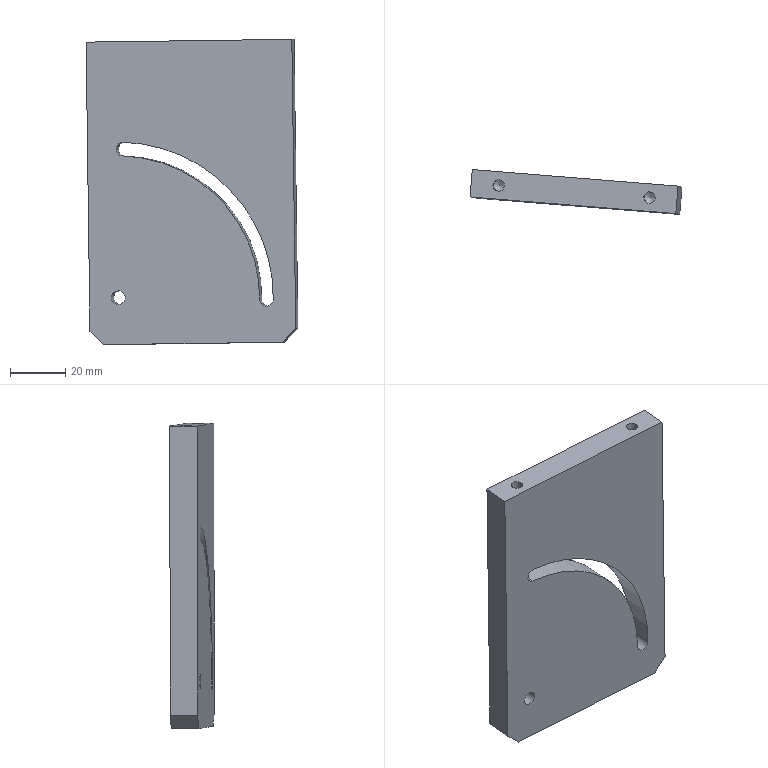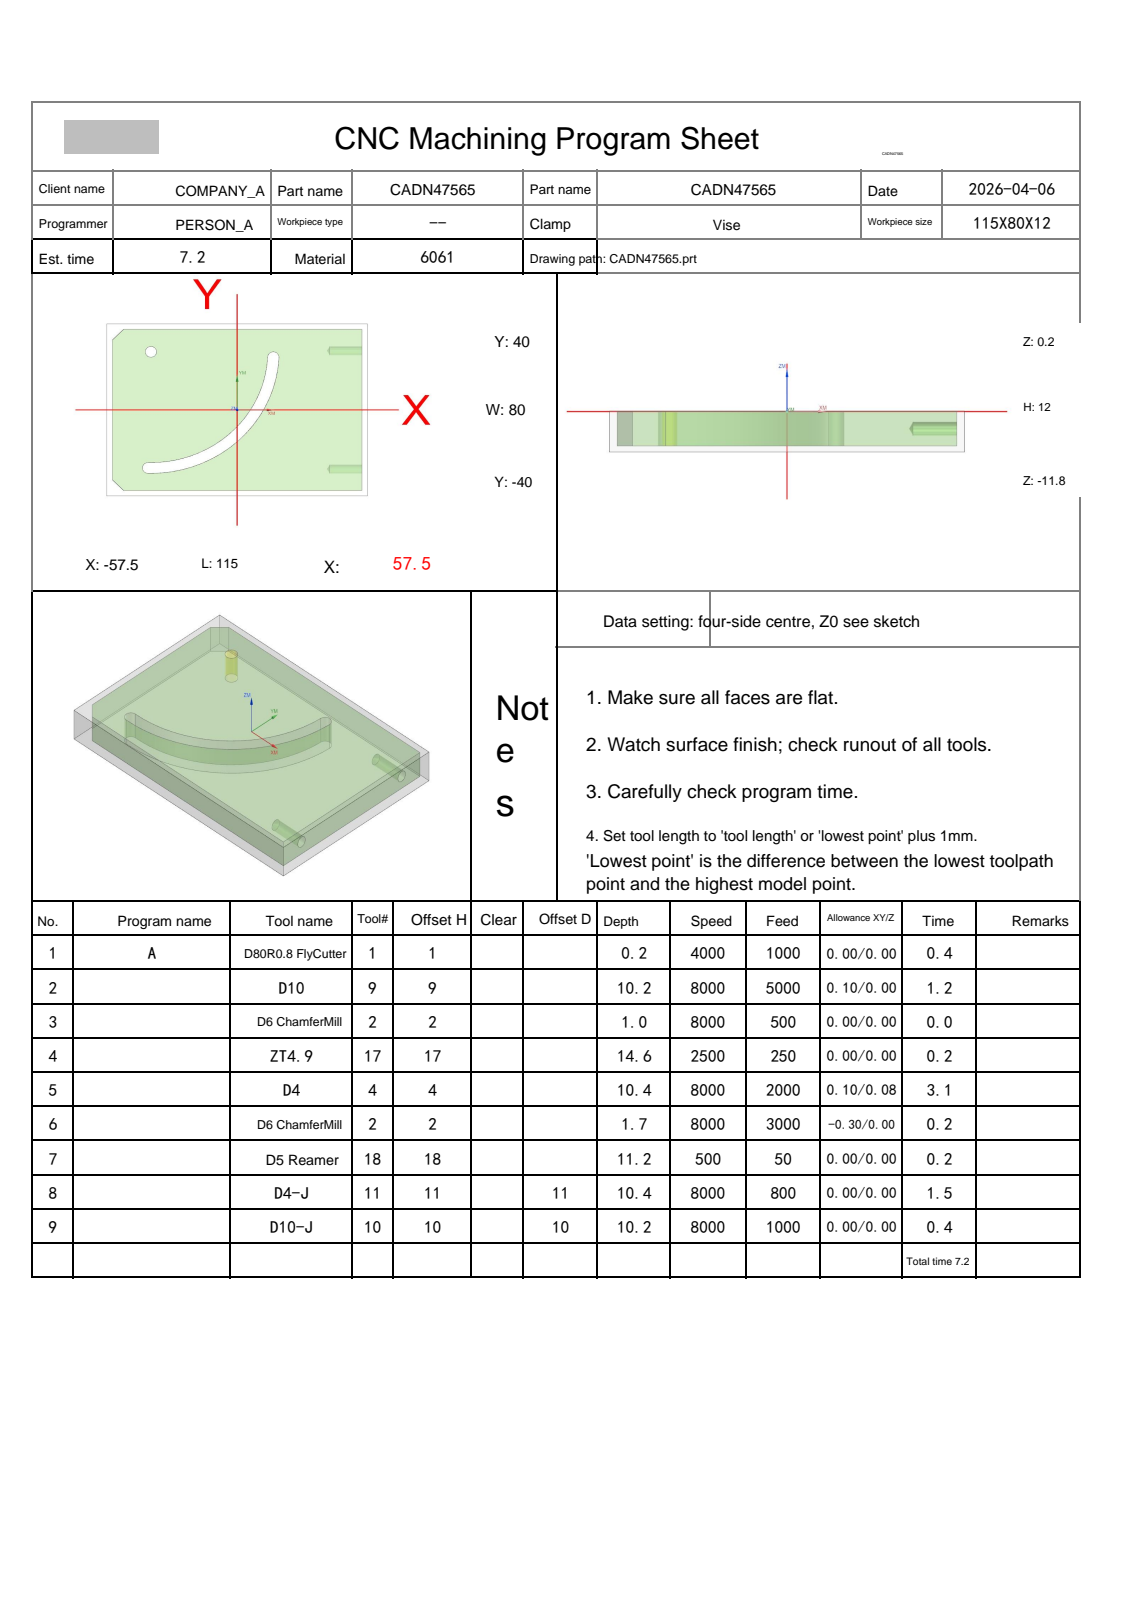NC program | NX | posted by the shop | part box 76.959 x 16.139 x 110.936 mm
Whole program:
%
O0001
(Machine time: 9.16 MIN)
(===Total Tool:8===)
(T1=D80R0.8 FlyCutter D=80.  R=0.8  D-  H01 Z=0.    )
(T9=D10     D=10.  R=0.   D-  H09 Z=-10.  )
(T2=D6 ChamferMill D=6.   R=0.   D-  H02 Z=-1.5  )
(T17=ZT4.9  D=4.9  DR_a=120 D-  H17 Z=-14.41)
(T4=D4      D=4.   R=0.   D-  H04 Z=-10.2 )
(T18=D5 Reamer D=5.   DR_a=180 D-  H18 Z=-11.  )
(T11=D4-J   D=4.   R=0.   D11 H11 Z=-10.2 )
(T10=D10-J  D=10.  R=0.   D10 H10 Z=-10.  )
G80 G90 G17 G49 G40
G91 G28 Z0
M01
N1 T01 M06
(D80R0.8 FlyCutter D=80. R=0.8 H=01 ce=0.00 di=0.00)
(MAX_Z=20. MIN_Z=0. Time=0.46M)
G00 G90 G54 X-100. Y25.833 M03 S4000
G43 H01 Z20.
M08
Z2.
G01 Z0.0 F1000.
X-95.
X95.
Y-25.833
X-95.
X-100.
Z2.
G00 Z20.
G91 G28 Z0.0
M05
M09
G91 G28 Z0.0
M01
N2 T09 M06
(D10  D=10. R=0. H=09 ce=0.10 di=0.00)
(MAX_Z=20. MIN_Z=-10. Time=1.20M)
G00 G90 G54 X2.5 Y42.6 M03 S8000
G43 H09 Z20.
M08
Z.5
G01 X55. Z.401 F5000.
G02 X60.1 Y37.5 Z.385 I0.0 J-5.1
G01 Y-37.5 Z.243
G02 X55. Y-42.6 Z.228 I-5.1 J0.0
G01 X-50. Z.03
G02 X-53.606 Y-41.106 Z.022 I0.0 J5.1
G01 X-58.606 Y-36.106 Z.009
G02 X-60.1 Y-32.5 Z.001 I3.606 J3.606
G01 Y32.5 Z-.122
G02 X-58.606 Y36.106 Z-.13 I5.1 J0.0
G01 X-53.606 Y41.106 Z-.143
G02 X-50. Y42.6 Z-.151 I3.606 J-3.606
G01 X55. Z-.349
G02 X60.1 Y37.5 Z-.365 I0.0 J-5.1
G01 Y-37.5 Z-.507
G02 X55. Y-42.6 Z-.522 I-5.1 J0.0
G01 X-50. Z-.72
G02 X-53.606 Y-41.106 Z-.728 I0.0 J5.1
G01 X-58.606 Y-36.106 Z-.741
G02 X-60.1 Y-32.5 Z-.749 I3.606 J3.606
G01 Y32.5 Z-.872
G02 X-58.606 Y36.106 Z-.88 I5.1 J0.0
G01 X-53.606 Y41.106 Z-.893
G02 X-50. Y42.6 Z-.901 I3.606 J-3.606
G01 X55. Z-1.099
G02 X60.1 Y37.5 Z-1.115 I0.0 J-5.1
G01 Y-37.5 Z-1.257
G02 X55. Y-42.6 Z-1.272 I-5.1 J0.0
G01 X-50. Z-1.47
G02 X-53.606 Y-41.106 Z-1.478 I0.0 J5.1
G01 X-58.606 Y-36.106 Z-1.491
G02 X-60.1 Y-32.5 Z-1.499 I3.606 J3.606
G01 Y32.5 Z-1.622
G02 X-58.606 Y36.106 Z-1.63 I5.1 J0.0
G01 X-53.606 Y41.106 Z-1.643
G02 X-50. Y42.6 Z-1.651 I3.606 J-3.606
G01 X55. Z-1.849
G02 X60.1 Y37.5 Z-1.865 I0.0 J-5.1
G01 Y-37.5 Z-2.007
G02 X55. Y-42.6 Z-2.022 I-5.1 J0.0
G01 X-50. Z-2.22
G02 X-53.606 Y-41.106 Z-2.228 I0.0 J5.1
G01 X-58.606 Y-36.106 Z-2.241
G02 X-60.1 Y-32.5 Z-2.249 I3.606 J3.606
G01 Y32.5 Z-2.372
G02 X-58.606 Y36.106 Z-2.38 I5.1 J0.0
G01 X-53.606 Y41.106 Z-2.393
G02 X-50. Y42.6 Z-2.401 I3.606 J-3.606
G01 X55. Z-2.599
G02 X60.1 Y37.5 Z-2.615 I0.0 J-5.1
G01 Y-37.5 Z-2.757
G02 X55. Y-42.6 Z-2.772 I-5.1 J0.0
G01 X-50. Z-2.97
G02 X-53.606 Y-41.106 Z-2.978 I0.0 J5.1
G01 X-58.606 Y-36.106 Z-2.991
G02 X-60.1 Y-32.5 Z-2.999 I3.606 J3.606
G01 Y32.5 Z-3.122
G02 X-58.606 Y36.106 Z-3.13 I5.1 J0.0
G01 X-53.606 Y41.106 Z-3.143
G02 X-50. Y42.6 Z-3.151 I3.606 J-3.606
G01 X55. Z-3.349
G02 X60.1 Y37.5 Z-3.365 I0.0 J-5.1
G01 Y-37.5 Z-3.507
G02 X55. Y-42.6 Z-3.522 I-5.1 J0.0
G01 X-50. Z-3.72
G02 X-53.606 Y-41.106 Z-3.728 I0.0 J5.1
G01 X-58.606 Y-36.106 Z-3.741
G02 X-60.1 Y-32.5 Z-3.749 I3.606 J3.606
G01 Y32.5 Z-3.872
G02 X-58.606 Y36.106 Z-3.88 I5.1 J0.0
G01 X-53.606 Y41.106 Z-3.893
G02 X-50. Y42.6 Z-3.901 I3.606 J-3.606
G01 X55. Z-4.099
G02 X60.1 Y37.5 Z-4.115 I0.0 J-5.1
G01 Y-37.5 Z-4.257
G02 X55. Y-42.6 Z-4.272 I-5.1 J0.0
G01 X-50. Z-4.47
G02 X-53.606 Y-41.106 Z-4.478 I0.0 J5.1
G01 X-58.606 Y-36.106 Z-4.491
G02 X-60.1 Y-32.5 Z-4.499 I3.606 J3.606
G01 Y32.5 Z-4.622
G02 X-58.606 Y36.106 Z-4.63 I5.1 J0.0
G01 X-53.606 Y41.106 Z-4.643
G02 X-50. Y42.6 Z-4.651 I3.606 J-3.606
G01 X55. Z-4.849
G02 X60.1 Y37.5 Z-4.865 I0.0 J-5.1
G01 Y-37.5 Z-5.007
G02 X55. Y-42.6 Z-5.022 I-5.1 J0.0
G01 X-50. Z-5.22
G02 X-53.606 Y-41.106 Z-5.228 I0.0 J5.1
G01 X-58.606 Y-36.106 Z-5.241
G02 X-60.1 Y-32.5 Z-5.249 I3.606 J3.606
G01 Y32.5 Z-5.372
G02 X-58.606 Y36.106 Z-5.38 I5.1 J0.0
G01 X-53.606 Y41.106 Z-5.393
G02 X-50. Y42.6 Z-5.401 I3.606 J-3.606
G01 X55. Z-5.599
G02 X60.1 Y37.5 Z-5.615 I0.0 J-5.1
G01 Y-37.5 Z-5.757
G02 X55. Y-42.6 Z-5.772 I-5.1 J0.0
G01 X-50. Z-5.97
G02 X-53.606 Y-41.106 Z-5.978 I0.0 J5.1
G01 X-58.606 Y-36.106 Z-5.991
G02 X-60.1 Y-32.5 Z-5.999 I3.606 J3.606
G01 Y32.5 Z-6.122
G02 X-58.606 Y36.106 Z-6.13 I5.1 J0.0
G01 X-53.606 Y41.106 Z-6.143
G02 X-50. Y42.6 Z-6.151 I3.606 J-3.606
G01 X55. Z-6.349
G02 X60.1 Y37.5 Z-6.365 I0.0 J-5.1
G01 Y-37.5 Z-6.507
G02 X55. Y-42.6 Z-6.522 I-5.1 J0.0
G01 X-50. Z-6.72
G02 X-53.606 Y-41.106 Z-6.728 I0.0 J5.1
G01 X-58.606 Y-36.106 Z-6.741
G02 X-60.1 Y-32.5 Z-6.749 I3.606 J3.606
G01 Y32.5 Z-6.872
G02 X-58.606 Y36.106 Z-6.88 I5.1 J0.0
G01 X-53.606 Y41.106 Z-6.893
G02 X-50. Y42.6 Z-6.901 I3.606 J-3.606
G01 X55. Z-7.099
G02 X60.1 Y37.5 Z-7.115 I0.0 J-5.1
G01 Y-37.5 Z-7.257
G02 X55. Y-42.6 Z-7.272 I-5.1 J0.0
G01 X-50. Z-7.47
G02 X-53.606 Y-41.106 Z-7.478 I0.0 J5.1
G01 X-58.606 Y-36.106 Z-7.491
G02 X-60.1 Y-32.5 Z-7.499 I3.606 J3.606
G01 Y32.5 Z-7.622
G02 X-58.606 Y36.106 Z-7.63 I5.1 J0.0
G01 X-53.606 Y41.106 Z-7.643
G02 X-50. Y42.6 Z-7.651 I3.606 J-3.606
G01 X55. Z-7.849
G02 X60.1 Y37.5 Z-7.865 I0.0 J-5.1
G01 Y-37.5 Z-8.007
G02 X55. Y-42.6 Z-8.022 I-5.1 J0.0
G01 X-50. Z-8.22
G02 X-53.606 Y-41.106 Z-8.228 I0.0 J5.1
G01 X-58.606 Y-36.106 Z-8.241
G02 X-60.1 Y-32.5 Z-8.249 I3.606 J3.606
G01 Y32.5 Z-8.372
G02 X-58.606 Y36.106 Z-8.38 I5.1 J0.0
G01 X-53.606 Y41.106 Z-8.393
G02 X-50. Y42.6 Z-8.401 I3.606 J-3.606
G01 X55. Z-8.599
G02 X60.1 Y37.5 Z-8.615 I0.0 J-5.1
G01 Y-37.5 Z-8.757
G02 X55. Y-42.6 Z-8.772 I-5.1 J0.0
G01 X-50. Z-8.97
G02 X-53.606 Y-41.106 Z-8.978 I0.0 J5.1
G01 X-58.606 Y-36.106 Z-8.991
G02 X-60.1 Y-32.5 Z-8.999 I3.606 J3.606
G01 Y32.5 Z-9.122
G02 X-58.606 Y36.106 Z-9.13 I5.1 J0.0
G01 X-53.606 Y41.106 Z-9.143
G02 X-50. Y42.6 Z-9.151 I3.606 J-3.606
G01 X55. Z-9.349
G02 X60.1 Y37.5 Z-9.365 I0.0 J-5.1
G01 Y-37.5 Z-9.507
G02 X55. Y-42.6 Z-9.522 I-5.1 J0.0
G01 X-50. Z-9.72
G02 X-53.606 Y-41.106 Z-9.728 I0.0 J5.1
G01 X-58.606 Y-36.106 Z-9.741
G02 X-60.1 Y-32.5 Z-9.749 I3.606 J3.606
G01 Y32.5 Z-9.872
G02 X-58.606 Y36.106 Z-9.88 I5.1 J0.0
G01 X-53.606 Y41.106 Z-9.893
G02 X-50. Y42.6 Z-9.901 I3.606 J-3.606
G01 X2.5 Z-10.
X55.
G02 X60.1 Y37.5 I0.0 J-5.1
G01 Y-37.5
G02 X55. Y-42.6 I-5.1 J0.0
G01 X-50.
G02 X-53.606 Y-41.106 I0.0 J5.1
G01 X-58.606 Y-36.106
G02 X-60.1 Y-32.5 I3.606 J3.606
G01 Y32.5
G02 X-58.606 Y36.106 I5.1 J0.0
G01 X-53.606 Y41.106
G02 X-50. Y42.6 I3.606 J-3.606
G01 X2.5
X3.
Z-9.
G00 Z20.
G91 G28 Z0.0
M05
M09
G91 G28 Z0.0
M01
N3 T02 M06
(D6 ChamferMill D=6. R=0. H=02 ce=0.00 di=0.00)
(MAX_Z=20. MIN_Z=-0.8 Time=0.03M)
G00 G90 G54 X-38. Y27. M03 S8000
G43 H02 Z20.
M08
G98 G81 X-38. Y27. Z-.8 R1. F500.
X-39.287 Y-26.985
X15.942 Y24.5
G80
G00 Z20.
G91 G28 Z0.0
M05
M09
G91 G28 Z0.0
M01
N4 T17 M06
(ZT4.9 D=4.9 DR_a=120 H=17)
(MAX_Z=20. MIN_Z=-14.41 Time=0.20M)
G00 G90 G54 X-38. Y27. M03 S2500
G43 H17 Z20.
M08
G98 G83 X-38. Y27. Z-14.415 R1. F250. Q2.
X-39.287 Y-26.985
X15.942 Y24.5
G80
G00 Z20.
G91 G28 Z0.0
M05
M09
G91 G28 Z0.0
M01
N5 T04 M06
(D4  D=4. R=0. H=04 ce=0.10 di=0.08)
(MAX_Z=20. MIN_Z=-10.2 Time=3.07M)
G00 G90 G54 X-25.456 Y-25.084 M03 S8000
G43 H04 Z20.
M08
Z.8
G01 X-27.62 Y-25.616 Z.683 F2000.
X-32.529 Y-26.35 Z.423
X-37.485 Y-26.628 Z.163
X-39.278 Y-26.585 Z.069
X-39.436 Y-26.581 Z.061
X-39.683 Y-26.817 Z.043
X-39.687 Y-26.975 Z.034
X-39.691 Y-27.133 Z.026
X-39.455 Y-27.381 Z.008
X-39.297 Y-27.385 Z0.0
G03 X16.342 Y24.481 Z-.145 I1.297 J54.385
X16.2 Y24.805 Z-.145 I-.4 J.019
X15.961 Y24.899 Z-.146 I-.258 J-.306
X15.543 Y24.518 Z-.147 I-.019 J-.4
G02 X-39.278 Y-26.585 Z-.289 I-53.543 J2.482
G03 X-39.687 Y-26.975 Z-.29 I-.01 J-.4
X-39.297 Y-27.385 Z-.291 I.4 J-.01
X16.342 Y24.481 Z-.436 I1.297 J54.385
X16.2 Y24.805 Z-.437 I-.4 J.019
X15.961 Y24.899 Z-.437 I-.258 J-.306
X15.543 Y24.518 Z-.438 I-.019 J-.4
G02 X-39.278 Y-26.585 Z-.581 I-53.543 J2.482
G03 X-39.687 Y-26.975 Z-.582 I-.01 J-.4
X-39.297 Y-27.385 Z-.583 I.4 J-.01
X16.342 Y24.481 Z-.727 I1.297 J54.385
X16.2 Y24.805 Z-.728 I-.4 J.019
X15.961 Y24.899 Z-.729 I-.258 J-.306
X15.543 Y24.518 Z-.73 I-.019 J-.4
G02 X-39.278 Y-26.585 Z-.872 I-53.543 J2.482
G03 X-39.687 Y-26.975 Z-.873 I-.01 J-.4
X-39.297 Y-27.385 Z-.874 I.4 J-.01
X16.342 Y24.481 Z-1.019 I1.297 J54.385
X16.2 Y24.805 Z-1.02 I-.4 J.019
X15.961 Y24.899 Z-1.02 I-.258 J-.306
X15.543 Y24.518 Z-1.021 I-.019 J-.4
G02 X-39.278 Y-26.585 Z-1.164 I-53.543 J2.482
G03 X-39.687 Y-26.975 Z-1.165 I-.01 J-.4
X-39.297 Y-27.385 Z-1.166 I.4 J-.01
X16.342 Y24.481 Z-1.31 I1.297 J54.385
X16.2 Y24.805 Z-1.311 I-.4 J.019
X15.961 Y24.899 Z-1.311 I-.258 J-.306
X15.543 Y24.518 Z-1.312 I-.019 J-.4
G02 X-39.278 Y-26.585 Z-1.455 I-53.543 J2.482
G03 X-39.687 Y-26.975 Z-1.456 I-.01 J-.4
X-39.297 Y-27.385 Z-1.457 I.4 J-.01
X16.342 Y24.481 Z-1.602 I1.297 J54.385
X16.2 Y24.805 Z-1.602 I-.4 J.019
X15.961 Y24.899 Z-1.603 I-.258 J-.306
X15.543 Y24.518 Z-1.604 I-.019 J-.4
G02 X-39.278 Y-26.585 Z-1.746 I-53.543 J2.482
G03 X-39.687 Y-26.975 Z-1.747 I-.01 J-.4
X-39.297 Y-27.385 Z-1.749 I.4 J-.01
X16.342 Y24.481 Z-1.893 I1.297 J54.385
X16.2 Y24.805 Z-1.894 I-.4 J.019
X15.961 Y24.899 Z-1.894 I-.258 J-.306
X15.543 Y24.518 Z-1.895 I-.019 J-.4
G02 X-39.278 Y-26.585 Z-2.038 I-53.543 J2.482
G03 X-39.687 Y-26.975 Z-2.039 I-.01 J-.4
X-39.297 Y-27.385 Z-2.04 I.4 J-.01
X16.342 Y24.481 Z-2.185 I1.297 J54.385
X16.2 Y24.805 Z-2.185 I-.4 J.019
X15.961 Y24.899 Z-2.186 I-.258 J-.306
X15.543 Y24.518 Z-2.187 I-.019 J-.4
G02 X-39.278 Y-26.585 Z-2.329 I-53.543 J2.482
G03 X-39.687 Y-26.975 Z-2.33 I-.01 J-.4
X-39.297 Y-27.385 Z-2.331 I.4 J-.01
X16.342 Y24.481 Z-2.476 I1.297 J54.385
X16.2 Y24.805 Z-2.477 I-.4 J.019
X15.961 Y24.899 Z-2.477 I-.258 J-.306
X15.543 Y24.518 Z-2.478 I-.019 J-.4
G02 X-39.278 Y-26.585 Z-2.621 I-53.543 J2.482
G03 X-39.687 Y-26.975 Z-2.622 I-.01 J-.4
X-39.297 Y-27.385 Z-2.623 I.4 J-.01
X16.342 Y24.481 Z-2.767 I1.297 J54.385
X16.2 Y24.805 Z-2.768 I-.4 J.019
X15.961 Y24.899 Z-2.769 I-.258 J-.306
X15.543 Y24.518 Z-2.77 I-.019 J-.4
G02 X-39.278 Y-26.585 Z-2.912 I-53.543 J2.482
G03 X-39.687 Y-26.975 Z-2.913 I-.01 J-.4
X-39.297 Y-27.385 Z-2.914 I.4 J-.01
X16.342 Y24.481 Z-3.059 I1.297 J54.385
X16.2 Y24.805 Z-3.06 I-.4 J.019
X15.961 Y24.899 Z-3.06 I-.258 J-.306
X15.543 Y24.518 Z-3.061 I-.019 J-.4
G02 X-39.278 Y-26.585 Z-3.204 I-53.543 J2.482
G03 X-39.687 Y-26.975 Z-3.205 I-.01 J-.4
X-39.297 Y-27.385 Z-3.206 I.4 J-.01
X16.342 Y24.481 Z-3.35 I1.297 J54.385
X16.2 Y24.805 Z-3.351 I-.4 J.019
X15.961 Y24.899 Z-3.351 I-.258 J-.306
X15.543 Y24.518 Z-3.352 I-.019 J-.4
G02 X-39.278 Y-26.585 Z-3.495 I-53.543 J2.482
G03 X-39.687 Y-26.975 Z-3.496 I-.01 J-.4
X-39.297 Y-27.385 Z-3.497 I.4 J-.01
X16.342 Y24.481 Z-3.642 I1.297 J54.385
X16.2 Y24.805 Z-3.642 I-.4 J.019
X15.961 Y24.899 Z-3.643 I-.258 J-.306
X15.543 Y24.518 Z-3.644 I-.019 J-.4
G02 X-39.278 Y-26.585 Z-3.786 I-53.543 J2.482
G03 X-39.687 Y-26.975 Z-3.787 I-.01 J-.4
X-39.297 Y-27.385 Z-3.789 I.4 J-.01
X16.342 Y24.481 Z-3.933 I1.297 J54.385
X16.2 Y24.805 Z-3.934 I-.4 J.019
X15.961 Y24.899 Z-3.934 I-.258 J-.306
X15.543 Y24.518 Z-3.935 I-.019 J-.4
G02 X-39.278 Y-26.585 Z-4.078 I-53.543 J2.482
G03 X-39.687 Y-26.975 Z-4.079 I-.01 J-.4
X-39.297 Y-27.385 Z-4.08 I.4 J-.01
X16.342 Y24.481 Z-4.225 I1.297 J54.385
X16.2 Y24.805 Z-4.225 I-.4 J.019
X15.961 Y24.899 Z-4.226 I-.258 J-.306
X15.543 Y24.518 Z-4.227 I-.019 J-.4
G02 X-39.278 Y-26.585 Z-4.369 I-53.543 J2.482
G03 X-39.687 Y-26.975 Z-4.37 I-.01 J-.4
X-39.297 Y-27.385 Z-4.371 I.4 J-.01
X16.342 Y24.481 Z-4.516 I1.297 J54.385
X16.2 Y24.805 Z-4.517 I-.4 J.019
X15.961 Y24.899 Z-4.517 I-.258 J-.306
X15.543 Y24.518 Z-4.518 I-.019 J-.4
G02 X-39.278 Y-26.585 Z-4.661 I-53.543 J2.482
G03 X-39.687 Y-26.975 Z-4.662 I-.01 J-.4
X-39.297 Y-27.385 Z-4.663 I.4 J-.01
X16.342 Y24.481 Z-4.807 I1.297 J54.385
X16.2 Y24.805 Z-4.808 I-.4 J.019
X15.961 Y24.899 Z-4.809 I-.258 J-.306
X15.543 Y24.518 Z-4.81 I-.019 J-.4
G02 X-39.278 Y-26.585 Z-4.952 I-53.543 J2.482
G03 X-39.687 Y-26.975 Z-4.953 I-.01 J-.4
X-39.297 Y-27.385 Z-4.954 I.4 J-.01
X16.342 Y24.481 Z-5.099 I1.297 J54.385
X16.2 Y24.805 Z-5.1 I-.4 J.019
X15.961 Y24.899 Z-5.1 I-.258 J-.306
X15.543 Y24.518 Z-5.101 I-.019 J-.4
G02 X-39.278 Y-26.585 Z-5.244 I-53.543 J2.482
G03 X-39.687 Y-26.975 Z-5.245 I-.01 J-.4
X-39.297 Y-27.385 Z-5.246 I.4 J-.01
X16.342 Y24.481 Z-5.39 I1.297 J54.385
X16.2 Y24.805 Z-5.391 I-.4 J.019
X15.961 Y24.899 Z-5.391 I-.258 J-.306
X15.543 Y24.518 Z-5.392 I-.019 J-.4
G02 X-39.278 Y-26.585 Z-5.535 I-53.543 J2.482
G03 X-39.687 Y-26.975 Z-5.536 I-.01 J-.4
X-39.297 Y-27.385 Z-5.537 I.4 J-.01
X16.342 Y24.481 Z-5.682 I1.297 J54.385
X16.2 Y24.805 Z-5.682 I-.4 J.019
X15.961 Y24.899 Z-5.683 I-.258 J-.306
X15.543 Y24.518 Z-5.684 I-.019 J-.4
G02 X-39.278 Y-26.585 Z-5.826 I-53.543 J2.482
G03 X-39.687 Y-26.975 Z-5.827 I-.01 J-.4
X-39.297 Y-27.385 Z-5.829 I.4 J-.01
X16.342 Y24.481 Z-5.973 I1.297 J54.385
X16.2 Y24.805 Z-5.974 I-.4 J.019
X15.961 Y24.899 Z-5.974 I-.258 J-.306
X15.543 Y24.518 Z-5.975 I-.019 J-.4
G02 X-39.278 Y-26.585 Z-6.118 I-53.543 J2.482
G03 X-39.687 Y-26.975 Z-6.119 I-.01 J-.4
X-39.297 Y-27.385 Z-6.12 I.4 J-.01
X16.342 Y24.481 Z-6.265 I1.297 J54.385
X16.2 Y24.805 Z-6.265 I-.4 J.019
X15.961 Y24.899 Z-6.266 I-.258 J-.306
X15.543 Y24.518 Z-6.267 I-.019 J-.4
G02 X-39.278 Y-26.585 Z-6.409 I-53.543 J2.482
G03 X-39.687 Y-26.975 Z-6.41 I-.01 J-.4
X-39.297 Y-27.385 Z-6.411 I.4 J-.01
X16.342 Y24.481 Z-6.556 I1.297 J54.385
X16.2 Y24.805 Z-6.557 I-.4 J.019
X15.961 Y24.899 Z-6.557 I-.258 J-.306
X15.543 Y24.518 Z-6.558 I-.019 J-.4
G02 X-39.278 Y-26.585 Z-6.701 I-53.543 J2.482
G03 X-39.687 Y-26.975 Z-6.702 I-.01 J-.4
X-39.297 Y-27.385 Z-6.703 I.4 J-.01
X16.342 Y24.481 Z-6.847 I1.297 J54.385
X16.2 Y24.805 Z-6.848 I-.4 J.019
X15.961 Y24.899 Z-6.849 I-.258 J-.306
X15.543 Y24.518 Z-6.85 I-.019 J-.4
G02 X-39.278 Y-26.585 Z-6.992 I-53.543 J2.482
G03 X-39.687 Y-26.975 Z-6.993 I-.01 J-.4
X-39.297 Y-27.385 Z-6.994 I.4 J-.01
X16.342 Y24.481 Z-7.139 I1.297 J54.385
X16.2 Y24.805 Z-7.14 I-.4 J.019
X15.961 Y24.899 Z-7.14 I-.258 J-.306
X15.543 Y24.518 Z-7.141 I-.019 J-.4
G02 X-39.278 Y-26.585 Z-7.284 I-53.543 J2.482
G03 X-39.687 Y-26.975 Z-7.285 I-.01 J-.4
X-39.297 Y-27.385 Z-7.286 I.4 J-.01
X16.342 Y24.481 Z-7.43 I1.297 J54.385
X16.2 Y24.805 Z-7.431 I-.4 J.019
X15.961 Y24.899 Z-7.431 I-.258 J-.306
X15.543 Y24.518 Z-7.432 I-.019 J-.4
G02 X-39.278 Y-26.585 Z-7.575 I-53.543 J2.482
G03 X-39.687 Y-26.975 Z-7.576 I-.01 J-.4
X-39.297 Y-27.385 Z-7.577 I.4 J-.01
X16.342 Y24.481 Z-7.722 I1.297 J54.385
X16.2 Y24.805 Z-7.722 I-.4 J.019
X15.961 Y24.899 Z-7.723 I-.258 J-.306
X15.543 Y24.518 Z-7.724 I-.019 J-.4
G02 X-39.278 Y-26.585 Z-7.866 I-53.543 J2.482
G03 X-39.687 Y-26.975 Z-7.867 I-.01 J-.4
X-39.297 Y-27.385 Z-7.869 I.4 J-.01
X16.342 Y24.481 Z-8.013 I1.297 J54.385
X16.2 Y24.805 Z-8.014 I-.4 J.019
X15.961 Y24.899 Z-8.014 I-.258 J-.306
X15.543 Y24.518 Z-8.015 I-.019 J-.4
G02 X-39.278 Y-26.585 Z-8.158 I-53.543 J2.482
G03 X-39.687 Y-26.975 Z-8.159 I-.01 J-.4
X-39.297 Y-27.385 Z-8.16 I.4 J-.01
X16.342 Y24.481 Z-8.305 I1.297 J54.385
X16.2 Y24.805 Z-8.305 I-.4 J.019
X15.961 Y24.899 Z-8.306 I-.258 J-.306
X15.543 Y24.518 Z-8.307 I-.019 J-.4
G02 X-39.278 Y-26.585 Z-8.449 I-53.543 J2.482
G03 X-39.687 Y-26.975 Z-8.45 I-.01 J-.4
X-39.297 Y-27.385 Z-8.451 I.4 J-.01
X16.342 Y24.481 Z-8.596 I1.297 J54.385
X16.2 Y24.805 Z-8.597 I-.4 J.019
X15.961 Y24.899 Z-8.597 I-.258 J-.306
X15.543 Y24.518 Z-8.598 I-.019 J-.4
G02 X-39.278 Y-26.585 Z-8.741 I-53.543 J2.482
G03 X-39.687 Y-26.975 Z-8.742 I-.01 J-.4
X-39.297 Y-27.385 Z-8.743 I.4 J-.01
X16.342 Y24.481 Z-8.887 I1.297 J54.385
X16.2 Y24.805 Z-8.888 I-.4 J.019
X15.961 Y24.899 Z-8.889 I-.258 J-.306
X15.543 Y24.518 Z-8.89 I-.019 J-.4
G02 X-39.278 Y-26.585 Z-9.032 I-53.543 J2.482
G03 X-39.687 Y-26.975 Z-9.033 I-.01 J-.4
X-39.297 Y-27.385 Z-9.034 I.4 J-.01
X16.342 Y24.481 Z-9.179 I1.297 J54.385
X16.2 Y24.805 Z-9.18 I-.4 J.019
X15.961 Y24.899 Z-9.18 I-.258 J-.306
X15.543 Y24.518 Z-9.181 I-.019 J-.4
G02 X-39.278 Y-26.585 Z-9.324 I-53.543 J2.482
G03 X-39.687 Y-26.975 Z-9.325 I-.01 J-.4
X-39.297 Y-27.385 Z-9.326 I.4 J-.01
X16.342 Y24.481 Z-9.47 I1.297 J54.385
X16.2 Y24.805 Z-9.471 I-.4 J.019
X15.961 Y24.899 Z-9.471 I-.258 J-.306
X15.543 Y24.518 Z-9.472 I-.019 J-.4
G02 X-39.278 Y-26.585 Z-9.615 I-53.543 J2.482
G03 X-39.687 Y-26.975 Z-9.616 I-.01 J-.4
X-39.297 Y-27.385 Z-9.617 I.4 J-.01
X16.342 Y24.481 Z-9.762 I1.297 J54.385
X16.2 Y24.805 Z-9.762 I-.4 J.019
X15.961 Y24.899 Z-9.763 I-.258 J-.306
X15.543 Y24.518 Z-9.764 I-.019 J-.4
G02 X-39.278 Y-26.585 Z-9.906 I-53.543 J2.482
G03 X-39.687 Y-26.975 Z-9.907 I-.01 J-.4
X-39.297 Y-27.385 Z-9.909 I.4 J-.01
X16.342 Y24.481 Z-10.053 I1.297 J54.385
X16.2 Y24.805 Z-10.054 I-.4 J.019
X15.961 Y24.899 Z-10.054 I-.258 J-.306
X15.543 Y24.518 Z-10.055 I-.019 J-.4
G02 X-39.278 Y-26.585 Z-10.198 I-53.543 J2.482
G03 X-39.687 Y-26.975 Z-10.199 I-.01 J-.4
X-39.297 Y-27.385 Z-10.2 I.4 J-.01
X-38. Y-27.4 I1.297 J54.385
X16.342 Y24.481 I0.0 J54.4
G01 Y24.5
G03 X15.942 Y24.9 I-.4 J0.0
X15.543 Y24.518 I0.0 J-.4
G02 X-38. Y-26.6 I-53.543 J2.482
X-39.278 Y-26.585 I0.0 J53.6
G01 X-39.287
G03 X-39.687 Y-26.985 I0.0 J-.4
X-39.297 Y-27.385 I.4 J0.0
X-38.897 Y-27.393 I1.297 J54.385
G01 Z-9.4
G00 Z20.
G91 G28 Z0.0
M05
M09
G91 G28 Z0.0
M01
N6 T02 M06
(D6 ChamferMill D=6. R=0. H=02 ce=0.00 di=0.00)
(MAX_Z=20. MIN_Z=-1.5 Time=0.25M)
G00 G90 G54 X2.25 Y39.628 M03 S8000
G43 H02 Z20.
M08
Z2.099
G01 Z-1.499 F3000.
G03 X2.17 Y39.328 I.52 J-.3
X2.47 Y38.808 I.6 J0.0
G01 X2.5 Y38.8
X55.
G02 X56.3 Y37.5 I0.0 J-1.3
G01 Y-37.5
G02 X55. Y-38.8 I-1.3 J0.0
G01 X-50.
X-50.254 Y-38.775
X-50.497 Y-38.701
X-50.722 Y-38.581
X-50.919 Y-38.419
X-55.919 Y-33.419
X-56.081 Y-33.222
X-56.201 Y-32.997
X-56.275 Y-32.754
X-56.3 Y-32.5
Y32.5
X-56.275 Y32.754
X-56.201 Y32.997
X-56.081 Y33.222
X-55.919 Y33.419
X-50.919 Y38.419
X-50.722 Y38.581
X-50.497 Y38.701
X-50.254 Y38.775
X-50. Y38.8
X2.5
X2.53 Y38.808
G03 X2.83 Y39.328 I-.3 J.52
X2.75 Y39.628 I-.6 J0.0
G01 Z2.099
G00 Z20.
X-1.116 Y-12.956
Z2.109
G01 Z-1.499
G03 X-.534 Y-13.41 I.582 J.146
G01 X-.388 Y-13.392
X-.361 Y-13.377
G03 X17.141 Y24.444 I-37.639 J40.377
G01 X17.142 Y24.5
G03 X15.942 Y25.7 I-1.2 J0.0
X14.743 Y24.555 I0.0 J-1.2
G02 X-38. Y-25.8 I-52.743 J2.445
X-39.259 Y-25.785 I0.0 J52.8
G01 X-39.287
G03 X-40.487 Y-26.985 I0.0 J-1.2
X-39.316 Y-28.184 I1.2 J0.0
X-38. Y-28.2 I1.316 J55.184
X-.361 Y-13.377 I0.0 J55.2
G01 X-.344 Y-13.351
X-.314 Y-13.165
G03 X-.728 Y-12.595 I-.6 J0.0
G01 Z2.109
G00 Z20.
G00 G90 X-37.854 Y26.214 M03 S8000
Z20.
Z-.5
G01 Z-1. F500.
X-37.72 Y25.496
X-37.7
G03 X-36.2 Y26.976 I0.0 J1.5
G01 Y27.
G03 X-38. Y28.8 I-1.8 J0.0
X-39.8 Y27. I0.0 J-1.8
X-38. Y25.2 I1.8 J0.0
X-36.2 Y26.976 I0.0 J1.8
G01 Y26.996
G03 X-37.68 Y28.496 I-1.5 J0.0
G01 X-37.833 Y27.782
Z-.5
G00 Z20.
G91 G28 Z0.0
M05
M09
G91 G28 Z0.0
M01
N7 T18 M06
(D5 Reamer D=5. DR_a=180 H=18)
(MAX_Z=20. MIN_Z=-11. Time=0.24M)
G00 G90 G54 X-38. Y27. M03 S500
G43 H18 Z20.
M08
G98 G81 X-38. Y27. Z-11. R1. F50.
G80
G00 Z20.
G91 G28 Z0.0
M05
M09
G91 G28 Z0.0
M01
N8 T11 M06
(D4-J  D=4. R=0. H=11 ce=0.00 di=0.00)
(D.N=11 MAX_Z=20. MIN_Z=-10.2 Time=1.51M)
G00 G90 G54 X-31.192 Y-26.095 M03 S8000
G43 H11 Z20.
M08
Z.5
G01 X-32.447 Y-26.25 Z.434 F800.
X-34.476 Y-26.423 Z.327
X-36.509 Y-26.518 Z.22
X-38.545 Y-26.536 Z.114
X-39.276 Y-26.519 Z.075
X-39.345 Y-26.517 Z.072
X-39.389 Y-26.525 Z.069
X-39.453 Y-26.549 Z.066
X-39.517 Y-26.574 Z.062
X-39.627 Y-26.659 Z.055
X-39.708 Y-26.773 Z.048
X-39.752 Y-26.905 Z.04
X-39.753 Y-26.974 Z.037
X-39.755 Y-27.042 Z.033
X-39.695 Y-27.22 Z.023
X-39.571 Y-27.361 Z.013
X-39.402 Y-27.442 Z.004
X-39.334 Y-27.448 Z0.0
G41 D11
X-39.299 Y-27.485
G03 X16.442 Y24.476 Z-.842 I1.299 J54.485
X15.965 Y24.999 Z-.85 I-.499 J.023
X15.443 Y24.523 Z-.858 I-.023 J-.499
G02 X-39.275 Y-26.485 Z-1.684 I-53.443 J2.477
G01 X-39.34 Y-26.482 Z-1.685
X-39.405 Y-26.493 Z-1.686
X-39.465 Y-26.517
G03 X-39.787 Y-26.973 Z-1.692 I.178 J-.467
X-39.299 Y-27.485 Z-1.7 I.5 J-.012
X16.442 Y24.476 Z-2.542 I1.299 J54.485
X15.965 Y24.999 Z-2.55 I-.499 J.023
X15.443 Y24.523 Z-2.558 I-.023 J-.499
G02 X-39.275 Y-26.485 Z-3.384 I-53.443 J2.477
G01 X-39.34 Y-26.482 Z-3.385
X-39.405 Y-26.493 Z-3.386
X-39.465 Y-26.517
G03 X-39.787 Y-26.973 Z-3.392 I.178 J-.467
X-39.299 Y-27.485 Z-3.4 I.5 J-.012
X16.442 Y24.476 Z-4.242 I1.299 J54.485
X15.965 Y24.999 Z-4.25 I-.499 J.023
X15.443 Y24.523 Z-4.258 I-.023 J-.499
G02 X-39.275 Y-26.485 Z-5.084 I-53.443 J2.477
G01 X-39.34 Y-26.482 Z-5.085
X-39.405 Y-26.493 Z-5.086
X-39.465 Y-26.517
G03 X-39.787 Y-26.973 Z-5.092 I.178 J-.467
X-39.299 Y-27.485 Z-5.1 I.5 J-.012
X16.442 Y24.476 Z-5.942 I1.299 J54.485
X15.965 Y24.999 Z-5.95 I-.499 J.023
X15.443 Y24.523 Z-5.958 I-.023 J-.499
G02 X-39.275 Y-26.485 Z-6.784 I-53.443 J2.477
G01 X-39.34 Y-26.482 Z-6.785
X-39.405 Y-26.493 Z-6.786
X-39.465 Y-26.517
G03 X-39.787 Y-26.973 Z-6.792 I.178 J-.467
X-39.299 Y-27.485 Z-6.8 I.5 J-.012
X16.442 Y24.476 Z-7.642 I1.299 J54.485
X15.965 Y24.999 Z-7.65 I-.499 J.023
X15.443 Y24.523 Z-7.658 I-.023 J-.499
G02 X-39.275 Y-26.485 Z-8.484 I-53.443 J2.477
G01 X-39.34 Y-26.482 Z-8.485
X-39.405 Y-26.493 Z-8.486
X-39.465 Y-26.517
G03 X-39.787 Y-26.973 Z-8.492 I.178 J-.467
X-39.299 Y-27.485 Z-8.5 I.5 J-.012
X16.442 Y24.476 Z-9.342 I1.299 J54.485
X15.965 Y24.999 Z-9.35 I-.499 J.023
X15.443 Y24.523 Z-9.358 I-.023 J-.499
G02 X-39.275 Y-26.485 Z-10.184 I-53.443 J2.477
G01 X-39.34 Y-26.482 Z-10.185
X-39.405 Y-26.493 Z-10.186
X-39.465 Y-26.517
G03 X-39.787 Y-26.973 Z-10.192 I.178 J-.467
X-39.299 Y-27.485 Z-10.2 I.5 J-.012
X-38. Y-27.5 I1.299 J54.485
X16.442 Y24.476 I0.0 J54.5
G01 Y24.5
G03 X15.942 Y25. I-.5 J0.0
X15.443 Y24.523 I0.0 J-.5
G02 X-38. Y-26.5 I-53.443 J2.477
X-39.275 Y-26.485 I0.0 J53.5
G01 X-39.287
G03 X-39.787 Y-26.985 I0.0 J-.5
X-39.299 Y-27.485 I.5 J0.0
X-38.899 Y-27.493 I1.299 J54.485
G01 X-38.872 Y-27.491
X-38.851 Y-27.471
X-38.848 Y-27.443
G40 Y-27.393
Z-9.2
G00 Z20.
G91 G28 Z0.0
M05
M09
G91 G28 Z0.0
M01
N9 T10 M06
(D10-J  D=10. R=0. H=10 ce=0.00 di=0.00)
(D.N=10 MAX_Z=20. MIN_Z=-10. Time=0.41M)
G00 G90 G54 X-51.047 Y43.61 M03 S8000
G43 H10 Z20.
M08
Z-9.5
G01 Z-10. F1000.
G41 D10
X-51.029 Y43.411
G03 X-50.033 Y42.5 I.996 J.089
G01 X-50.027
X55.
G02 X60. Y37.5 I0.0 J-5.
G01 Y-37.5
G02 X55. Y-42.5 I-5. J0.0
G01 X-50.
G02 X-53.536 Y-41.036 I0.0 J5.
G01 X-58.536 Y-36.036
G02 X-60. Y-32.5 I3.536 J3.536
G01 Y32.5
G02 X-58.536 Y36.036 I5. J0.0
G01 X-53.536 Y41.036
G02 X-50.027 Y42.5 I3.536 J-3.536
G01 X-49.527
G03 X-48.527 Y43.5 I0.0 J1.
G01 G40 Y43.7
Z-9.5
G00 Z20.
M05
M09
G91 G28 Z0.0
G91 G28 Y0.0
M30
%